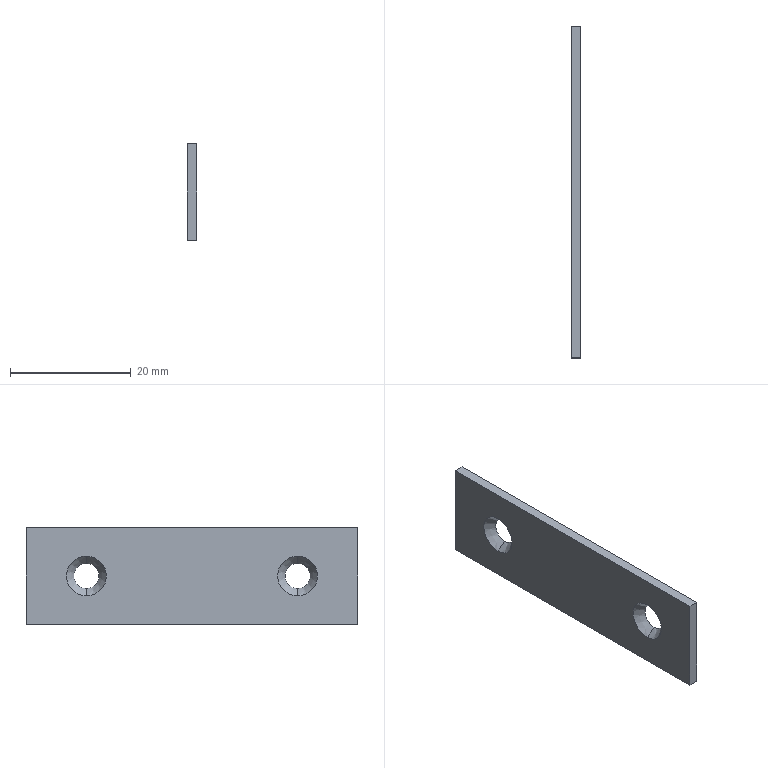Part | SolidWorks | features BaseBody 1 | 1 solid | 10 faces | box 1.6 x 55 x 16 mm | volume 1334 mm3 | plane 6 | cone 4
STEP:
#1=CARTESIAN_POINT('',(1.6,-17.5,2.1));
#2=VERTEX_POINT('',#1);
#3=CARTESIAN_POINT('',(1.6,-17.5,-2.1));
#4=VERTEX_POINT('',#3);
#5=CARTESIAN_POINT('',(1.6,-17.5,0.));
#6=DIRECTION('',(1.,0.,0.));
#7=DIRECTION('',(0.,0.,-1.));
#8=AXIS2_PLACEMENT_3D('',#5,#6,#7);
#9=CIRCLE('',#8,2.1);
#10=EDGE_CURVE('',#2,#4,#9,.T.);
#11=ORIENTED_EDGE('',*,*,#10,.T.);
#12=CARTESIAN_POINT('',(0.,-17.5,-3.3));
#13=VERTEX_POINT('',#12);
#14=CARTESIAN_POINT('',(0.,-17.5,-3.3));
#15=DIRECTION('',(-0.8,0.,-0.6));
#16=VECTOR('',#15,1000.);
#17=LINE('',#14,#16);
#18=EDGE_CURVE('',#4,#13,#17,.T.);
#19=ORIENTED_EDGE('',*,*,#18,.T.);
#20=CARTESIAN_POINT('',(0.,-17.5,3.3));
#21=VERTEX_POINT('',#20);
#22=CARTESIAN_POINT('',(0.,-17.5,0.));
#23=DIRECTION('',(1.,0.,0.));
#24=DIRECTION('',(0.,0.,-1.));
#25=AXIS2_PLACEMENT_3D('',#22,#23,#24);
#26=CIRCLE('',#25,3.3);
#27=EDGE_CURVE('',#21,#13,#26,.T.);
#28=ORIENTED_EDGE('',*,*,#27,.F.);
#29=CARTESIAN_POINT('',(0.,-17.5,3.3));
#30=DIRECTION('',(-0.8,0.,0.6));
#31=VECTOR('',#30,1000.);
#32=LINE('',#29,#31);
#33=EDGE_CURVE('',#2,#21,#32,.T.);
#34=ORIENTED_EDGE('',*,*,#33,.F.);
#35=EDGE_LOOP('',(#11,#19,#28,#34));
#36=FACE_OUTER_BOUND('',#35,.T.);
#37=CARTESIAN_POINT('',(0.,-17.5,0.));
#38=DIRECTION('',(-1.,0.,0.));
#39=DIRECTION('',(0.,0.,1.));
#40=AXIS2_PLACEMENT_3D('',#37,#38,#39);
#41=CONICAL_SURFACE('',#40,3.3,0.6435);
#42=ADVANCED_FACE('',(#36),#41,.F.);
#43=CARTESIAN_POINT('',(1.6,17.5,2.1));
#44=VERTEX_POINT('',#43);
#45=CARTESIAN_POINT('',(1.6,17.5,-2.1));
#46=VERTEX_POINT('',#45);
#47=CARTESIAN_POINT('',(1.6,17.5,0.));
#48=DIRECTION('',(1.,0.,0.));
#49=DIRECTION('',(0.,0.,-1.));
#50=AXIS2_PLACEMENT_3D('',#47,#48,#49);
#51=CIRCLE('',#50,2.1);
#52=EDGE_CURVE('',#44,#46,#51,.T.);
#53=ORIENTED_EDGE('',*,*,#52,.T.);
#54=CARTESIAN_POINT('',(0.,17.5,-3.3));
#55=VERTEX_POINT('',#54);
#56=CARTESIAN_POINT('',(0.,17.5,-3.3));
#57=DIRECTION('',(-0.8,0.,-0.6));
#58=VECTOR('',#57,1000.);
#59=LINE('',#56,#58);
#60=EDGE_CURVE('',#46,#55,#59,.T.);
#61=ORIENTED_EDGE('',*,*,#60,.T.);
#62=CARTESIAN_POINT('',(0.,17.5,3.3));
#63=VERTEX_POINT('',#62);
#64=CARTESIAN_POINT('',(0.,17.5,0.));
#65=DIRECTION('',(1.,0.,0.));
#66=DIRECTION('',(0.,0.,-1.));
#67=AXIS2_PLACEMENT_3D('',#64,#65,#66);
#68=CIRCLE('',#67,3.3);
#69=EDGE_CURVE('',#63,#55,#68,.T.);
#70=ORIENTED_EDGE('',*,*,#69,.F.);
#71=CARTESIAN_POINT('',(0.,17.5,3.3));
#72=DIRECTION('',(-0.8,0.,0.6));
#73=VECTOR('',#72,1000.);
#74=LINE('',#71,#73);
#75=EDGE_CURVE('',#44,#63,#74,.T.);
#76=ORIENTED_EDGE('',*,*,#75,.F.);
#77=EDGE_LOOP('',(#53,#61,#70,#76));
#78=FACE_OUTER_BOUND('',#77,.T.);
#79=CARTESIAN_POINT('',(0.,17.5,0.));
#80=DIRECTION('',(-1.,0.,0.));
#81=DIRECTION('',(0.,0.,1.));
#82=AXIS2_PLACEMENT_3D('',#79,#80,#81);
#83=CONICAL_SURFACE('',#82,3.3,0.6435);
#84=ADVANCED_FACE('',(#78),#83,.F.);
#85=CARTESIAN_POINT('',(0.,-27.5,-8.));
#86=VERTEX_POINT('',#85);
#87=CARTESIAN_POINT('',(0.,27.5,-8.));
#88=VERTEX_POINT('',#87);
#89=CARTESIAN_POINT('',(0.,-27.5,-8.));
#90=DIRECTION('',(0.,1.,0.));
#91=VECTOR('',#90,1000.);
#92=LINE('',#89,#91);
#93=EDGE_CURVE('',#86,#88,#92,.T.);
#94=ORIENTED_EDGE('',*,*,#93,.T.);
#95=CARTESIAN_POINT('',(1.6,27.5,-8.));
#96=VERTEX_POINT('',#95);
#97=CARTESIAN_POINT('',(1.6,27.5,-8.));
#98=DIRECTION('',(-1.,0.,0.));
#99=VECTOR('',#98,1000.);
#100=LINE('',#97,#99);
#101=EDGE_CURVE('',#96,#88,#100,.T.);
#102=ORIENTED_EDGE('',*,*,#101,.F.);
#103=CARTESIAN_POINT('',(1.6,-27.5,-8.));
#104=VERTEX_POINT('',#103);
#105=CARTESIAN_POINT('',(1.6,-27.5,-8.));
#106=DIRECTION('',(0.,1.,0.));
#107=VECTOR('',#106,1000.);
#108=LINE('',#105,#107);
#109=EDGE_CURVE('',#104,#96,#108,.T.);
#110=ORIENTED_EDGE('',*,*,#109,.F.);
#111=CARTESIAN_POINT('',(1.6,-27.5,-8.));
#112=DIRECTION('',(-1.,0.,0.));
#113=VECTOR('',#112,1000.);
#114=LINE('',#111,#113);
#115=EDGE_CURVE('',#104,#86,#114,.T.);
#116=ORIENTED_EDGE('',*,*,#115,.T.);
#117=EDGE_LOOP('',(#94,#102,#110,#116));
#118=FACE_OUTER_BOUND('',#117,.T.);
#119=CARTESIAN_POINT('',(1.6,-27.5,-8.));
#120=DIRECTION('',(0.,0.,1.));
#121=DIRECTION('',(1.,0.,0.));
#122=AXIS2_PLACEMENT_3D('',#119,#120,#121);
#123=PLANE('',#122);
#124=ADVANCED_FACE('',(#118),#123,.F.);
#125=CARTESIAN_POINT('',(0.,-27.5,8.));
#126=VERTEX_POINT('',#125);
#127=CARTESIAN_POINT('',(0.,-27.5,8.));
#128=DIRECTION('',(0.,0.,-1.));
#129=VECTOR('',#128,1000.);
#130=LINE('',#127,#129);
#131=EDGE_CURVE('',#126,#86,#130,.T.);
#132=ORIENTED_EDGE('',*,*,#131,.T.);
#133=ORIENTED_EDGE('',*,*,#115,.F.);
#134=CARTESIAN_POINT('',(1.6,-27.5,8.));
#135=VERTEX_POINT('',#134);
#136=CARTESIAN_POINT('',(1.6,-27.5,8.));
#137=DIRECTION('',(0.,0.,-1.));
#138=VECTOR('',#137,1000.);
#139=LINE('',#136,#138);
#140=EDGE_CURVE('',#135,#104,#139,.T.);
#141=ORIENTED_EDGE('',*,*,#140,.F.);
#142=CARTESIAN_POINT('',(1.6,-27.5,8.));
#143=DIRECTION('',(-1.,0.,0.));
#144=VECTOR('',#143,1000.);
#145=LINE('',#142,#144);
#146=EDGE_CURVE('',#135,#126,#145,.T.);
#147=ORIENTED_EDGE('',*,*,#146,.T.);
#148=EDGE_LOOP('',(#132,#133,#141,#147));
#149=FACE_OUTER_BOUND('',#148,.T.);
#150=CARTESIAN_POINT('',(1.6,-27.5,8.));
#151=DIRECTION('',(0.,1.,0.));
#152=DIRECTION('',(1.,0.,0.));
#153=AXIS2_PLACEMENT_3D('',#150,#151,#152);
#154=PLANE('',#153);
#155=ADVANCED_FACE('',(#149),#154,.F.);
#156=CARTESIAN_POINT('',(0.,27.5,8.));
#157=VERTEX_POINT('',#156);
#158=CARTESIAN_POINT('',(0.,27.5,8.));
#159=DIRECTION('',(0.,-1.,0.));
#160=VECTOR('',#159,1000.);
#161=LINE('',#158,#160);
#162=EDGE_CURVE('',#157,#126,#161,.T.);
#163=ORIENTED_EDGE('',*,*,#162,.T.);
#164=ORIENTED_EDGE('',*,*,#146,.F.);
#165=CARTESIAN_POINT('',(1.6,27.5,8.));
#166=VERTEX_POINT('',#165);
#167=CARTESIAN_POINT('',(1.6,27.5,8.));
#168=DIRECTION('',(0.,-1.,0.));
#169=VECTOR('',#168,1000.);
#170=LINE('',#167,#169);
#171=EDGE_CURVE('',#166,#135,#170,.T.);
#172=ORIENTED_EDGE('',*,*,#171,.F.);
#173=CARTESIAN_POINT('',(1.6,27.5,8.));
#174=DIRECTION('',(-1.,0.,0.));
#175=VECTOR('',#174,1000.);
#176=LINE('',#173,#175);
#177=EDGE_CURVE('',#166,#157,#176,.T.);
#178=ORIENTED_EDGE('',*,*,#177,.T.);
#179=EDGE_LOOP('',(#163,#164,#172,#178));
#180=FACE_OUTER_BOUND('',#179,.T.);
#181=CARTESIAN_POINT('',(1.6,27.5,8.));
#182=DIRECTION('',(0.,0.,-1.));
#183=DIRECTION('',(0.,-1.,0.));
#184=AXIS2_PLACEMENT_3D('',#181,#182,#183);
#185=PLANE('',#184);
#186=ADVANCED_FACE('',(#180),#185,.F.);
#187=CARTESIAN_POINT('',(0.,27.5,-8.));
#188=DIRECTION('',(0.,0.,1.));
#189=VECTOR('',#188,1000.);
#190=LINE('',#187,#189);
#191=EDGE_CURVE('',#88,#157,#190,.T.);
#192=ORIENTED_EDGE('',*,*,#191,.T.);
#193=ORIENTED_EDGE('',*,*,#177,.F.);
#194=CARTESIAN_POINT('',(1.6,27.5,-8.));
#195=DIRECTION('',(0.,0.,1.));
#196=VECTOR('',#195,1000.);
#197=LINE('',#194,#196);
#198=EDGE_CURVE('',#96,#166,#197,.T.);
#199=ORIENTED_EDGE('',*,*,#198,.F.);
#200=ORIENTED_EDGE('',*,*,#101,.T.);
#201=EDGE_LOOP('',(#192,#193,#199,#200));
#202=FACE_OUTER_BOUND('',#201,.T.);
#203=CARTESIAN_POINT('',(1.6,27.5,-8.));
#204=DIRECTION('',(0.,-1.,0.));
#205=DIRECTION('',(0.,0.,-1.));
#206=AXIS2_PLACEMENT_3D('',#203,#204,#205);
#207=PLANE('',#206);
#208=ADVANCED_FACE('',(#202),#207,.F.);
#209=ORIENTED_EDGE('',*,*,#27,.T.);
#210=CARTESIAN_POINT('',(0.,-17.5,0.));
#211=DIRECTION('',(1.,0.,0.));
#212=DIRECTION('',(0.,0.,-1.));
#213=AXIS2_PLACEMENT_3D('',#210,#211,#212);
#214=CIRCLE('',#213,3.3);
#215=EDGE_CURVE('',#13,#21,#214,.T.);
#216=ORIENTED_EDGE('',*,*,#215,.T.);
#217=EDGE_LOOP('',(#209,#216));
#218=FACE_BOUND('',#217,.T.);
#219=ORIENTED_EDGE('',*,*,#69,.T.);
#220=CARTESIAN_POINT('',(0.,17.5,0.));
#221=DIRECTION('',(1.,0.,0.));
#222=DIRECTION('',(0.,0.,-1.));
#223=AXIS2_PLACEMENT_3D('',#220,#221,#222);
#224=CIRCLE('',#223,3.3);
#225=EDGE_CURVE('',#55,#63,#224,.T.);
#226=ORIENTED_EDGE('',*,*,#225,.T.);
#227=EDGE_LOOP('',(#219,#226));
#228=FACE_BOUND('',#227,.T.);
#229=ORIENTED_EDGE('',*,*,#191,.F.);
#230=ORIENTED_EDGE('',*,*,#93,.F.);
#231=ORIENTED_EDGE('',*,*,#131,.F.);
#232=ORIENTED_EDGE('',*,*,#162,.F.);
#233=EDGE_LOOP('',(#229,#230,#231,#232));
#234=FACE_OUTER_BOUND('',#233,.T.);
#235=CARTESIAN_POINT('',(0.,0.,0.));
#236=DIRECTION('',(1.,0.,0.));
#237=DIRECTION('',(0.,1.,0.));
#238=AXIS2_PLACEMENT_3D('',#235,#236,#237);
#239=PLANE('',#238);
#240=ADVANCED_FACE('',(#218,#228,#234),#239,.F.);
#241=ORIENTED_EDGE('',*,*,#10,.F.);
#242=CARTESIAN_POINT('',(1.6,-17.5,0.));
#243=DIRECTION('',(1.,0.,0.));
#244=DIRECTION('',(0.,0.,-1.));
#245=AXIS2_PLACEMENT_3D('',#242,#243,#244);
#246=CIRCLE('',#245,2.1);
#247=EDGE_CURVE('',#4,#2,#246,.T.);
#248=ORIENTED_EDGE('',*,*,#247,.F.);
#249=EDGE_LOOP('',(#241,#248));
#250=FACE_BOUND('',#249,.T.);
#251=ORIENTED_EDGE('',*,*,#52,.F.);
#252=CARTESIAN_POINT('',(1.6,17.5,0.));
#253=DIRECTION('',(1.,0.,0.));
#254=DIRECTION('',(0.,0.,-1.));
#255=AXIS2_PLACEMENT_3D('',#252,#253,#254);
#256=CIRCLE('',#255,2.1);
#257=EDGE_CURVE('',#46,#44,#256,.T.);
#258=ORIENTED_EDGE('',*,*,#257,.F.);
#259=EDGE_LOOP('',(#251,#258));
#260=FACE_BOUND('',#259,.T.);
#261=ORIENTED_EDGE('',*,*,#198,.T.);
#262=ORIENTED_EDGE('',*,*,#171,.T.);
#263=ORIENTED_EDGE('',*,*,#140,.T.);
#264=ORIENTED_EDGE('',*,*,#109,.T.);
#265=EDGE_LOOP('',(#261,#262,#263,#264));
#266=FACE_OUTER_BOUND('',#265,.T.);
#267=CARTESIAN_POINT('',(1.6,0.,0.));
#268=DIRECTION('',(1.,0.,0.));
#269=DIRECTION('',(0.,1.,0.));
#270=AXIS2_PLACEMENT_3D('',#267,#268,#269);
#271=PLANE('',#270);
#272=ADVANCED_FACE('',(#250,#260,#266),#271,.T.);
#273=ORIENTED_EDGE('',*,*,#60,.F.);
#274=ORIENTED_EDGE('',*,*,#257,.T.);
#275=ORIENTED_EDGE('',*,*,#75,.T.);
#276=ORIENTED_EDGE('',*,*,#225,.F.);
#277=EDGE_LOOP('',(#273,#274,#275,#276));
#278=FACE_OUTER_BOUND('',#277,.T.);
#279=CARTESIAN_POINT('',(0.,17.5,0.));
#280=DIRECTION('',(-1.,0.,0.));
#281=DIRECTION('',(0.,0.,1.));
#282=AXIS2_PLACEMENT_3D('',#279,#280,#281);
#283=CONICAL_SURFACE('',#282,3.3,0.6435);
#284=ADVANCED_FACE('',(#278),#283,.F.);
#285=ORIENTED_EDGE('',*,*,#18,.F.);
#286=ORIENTED_EDGE('',*,*,#247,.T.);
#287=ORIENTED_EDGE('',*,*,#33,.T.);
#288=ORIENTED_EDGE('',*,*,#215,.F.);
#289=EDGE_LOOP('',(#285,#286,#287,#288));
#290=FACE_OUTER_BOUND('',#289,.T.);
#291=CARTESIAN_POINT('',(0.,-17.5,0.));
#292=DIRECTION('',(-1.,0.,0.));
#293=DIRECTION('',(0.,0.,1.));
#294=AXIS2_PLACEMENT_3D('',#291,#292,#293);
#295=CONICAL_SURFACE('',#294,3.3,0.6435);
#296=ADVANCED_FACE('',(#290),#295,.F.);
#297=CLOSED_SHELL('',(#42,#84,#124,#155,#186,#208,#240,#272,#284,#296));
#298=MANIFOLD_SOLID_BREP('',#297);
#299=CARTESIAN_POINT('',(0.,0.,0.));
#300=DIRECTION('',(0.,0.,1.));
#301=DIRECTION('',(1.,0.,0.));
#302=AXIS2_PLACEMENT_3D('',#299,#300,#301);
#303=(LENGTH_UNIT()NAMED_UNIT(*)SI_UNIT(.MILLI.,.METRE.));
#304=UNCERTAINTY_MEASURE_WITH_UNIT(LENGTH_MEASURE(0.00001),#303,'','');
#305=(NAMED_UNIT(*)PLANE_ANGLE_UNIT()SI_UNIT($,.RADIAN.));
#306=(NAMED_UNIT(*)SI_UNIT($,.STERADIAN.)SOLID_ANGLE_UNIT());
#307=(GEOMETRIC_REPRESENTATION_CONTEXT(3)GLOBAL_UNCERTAINTY_ASSIGNED_CONTEXT((#304))GLOBAL_UNIT_ASSIGNED_CONTEXT((#303,#305,#306))REPRESENTATION_CONTEXT('',''));
#308=ADVANCED_BREP_SHAPE_REPRESENTATION('',(#298,#302),#307);